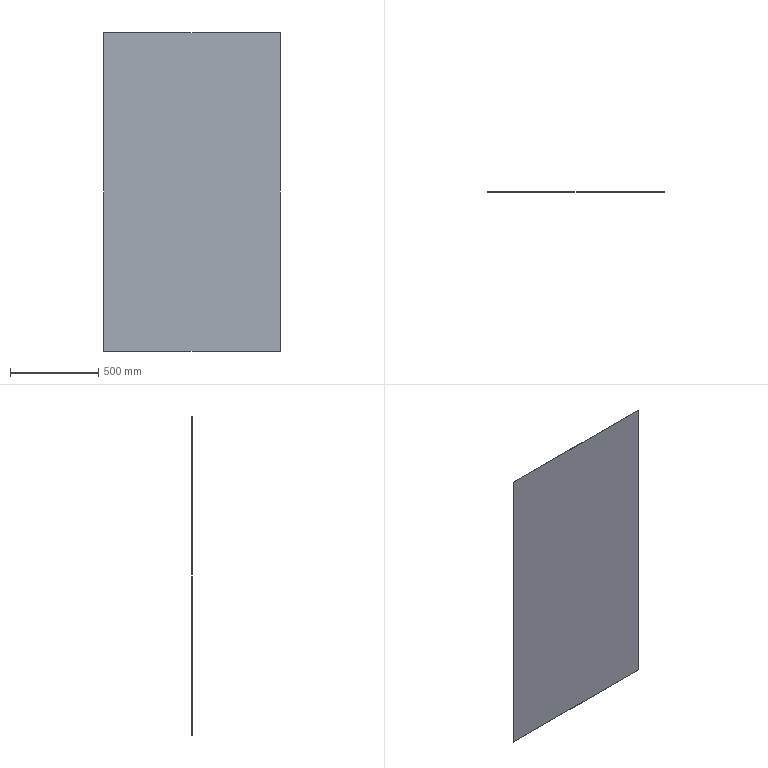Part | SolidWorks | features Extrusion 1 | 1 solid | 6 faces | box 1000 x 1 x 1800 mm | volume 1800000 mm3 | plane 6
STEP:
#1=CARTESIAN_POINT('',(500.,0.,900.));
#2=VERTEX_POINT('',#1);
#3=CARTESIAN_POINT('',(500.,0.,-900.));
#4=VERTEX_POINT('',#3);
#5=CARTESIAN_POINT('',(500.,0.,900.));
#6=DIRECTION('',(0.,0.,-1.));
#7=VECTOR('',#6,1000.);
#8=LINE('',#5,#7);
#9=EDGE_CURVE('',#2,#4,#8,.T.);
#10=ORIENTED_EDGE('',*,*,#9,.T.);
#11=CARTESIAN_POINT('',(500.,1.,-900.));
#12=VERTEX_POINT('',#11);
#13=CARTESIAN_POINT('',(500.,1.,-900.));
#14=DIRECTION('',(0.,-1.,0.));
#15=VECTOR('',#14,1000.);
#16=LINE('',#13,#15);
#17=EDGE_CURVE('',#12,#4,#16,.T.);
#18=ORIENTED_EDGE('',*,*,#17,.F.);
#19=CARTESIAN_POINT('',(500.,1.,900.));
#20=VERTEX_POINT('',#19);
#21=CARTESIAN_POINT('',(500.,1.,900.));
#22=DIRECTION('',(0.,0.,-1.));
#23=VECTOR('',#22,1000.);
#24=LINE('',#21,#23);
#25=EDGE_CURVE('',#20,#12,#24,.T.);
#26=ORIENTED_EDGE('',*,*,#25,.F.);
#27=CARTESIAN_POINT('',(500.,1.,900.));
#28=DIRECTION('',(0.,-1.,0.));
#29=VECTOR('',#28,1000.);
#30=LINE('',#27,#29);
#31=EDGE_CURVE('',#20,#2,#30,.T.);
#32=ORIENTED_EDGE('',*,*,#31,.T.);
#33=EDGE_LOOP('',(#10,#18,#26,#32));
#34=FACE_OUTER_BOUND('',#33,.T.);
#35=CARTESIAN_POINT('',(500.,1.,900.));
#36=DIRECTION('',(-1.,0.,0.));
#37=DIRECTION('',(0.,0.,1.));
#38=AXIS2_PLACEMENT_3D('',#35,#36,#37);
#39=PLANE('',#38);
#40=ADVANCED_FACE('',(#34),#39,.F.);
#41=CARTESIAN_POINT('',(-500.,0.,-900.));
#42=VERTEX_POINT('',#41);
#43=CARTESIAN_POINT('',(-500.,0.,-900.));
#44=DIRECTION('',(-1.,0.,0.));
#45=VECTOR('',#44,1000.);
#46=LINE('',#43,#45);
#47=EDGE_CURVE('',#4,#42,#46,.T.);
#48=ORIENTED_EDGE('',*,*,#47,.T.);
#49=CARTESIAN_POINT('',(-500.,1.,-900.));
#50=VERTEX_POINT('',#49);
#51=CARTESIAN_POINT('',(-500.,1.,-900.));
#52=DIRECTION('',(0.,-1.,0.));
#53=VECTOR('',#52,1000.);
#54=LINE('',#51,#53);
#55=EDGE_CURVE('',#50,#42,#54,.T.);
#56=ORIENTED_EDGE('',*,*,#55,.F.);
#57=CARTESIAN_POINT('',(-500.,1.,-900.));
#58=DIRECTION('',(-1.,0.,0.));
#59=VECTOR('',#58,1000.);
#60=LINE('',#57,#59);
#61=EDGE_CURVE('',#12,#50,#60,.T.);
#62=ORIENTED_EDGE('',*,*,#61,.F.);
#63=ORIENTED_EDGE('',*,*,#17,.T.);
#64=EDGE_LOOP('',(#48,#56,#62,#63));
#65=FACE_OUTER_BOUND('',#64,.T.);
#66=CARTESIAN_POINT('',(-500.,1.,-900.));
#67=DIRECTION('',(0.,0.,1.));
#68=DIRECTION('',(1.,0.,0.));
#69=AXIS2_PLACEMENT_3D('',#66,#67,#68);
#70=PLANE('',#69);
#71=ADVANCED_FACE('',(#65),#70,.F.);
#72=CARTESIAN_POINT('',(-500.,0.,900.));
#73=VERTEX_POINT('',#72);
#74=CARTESIAN_POINT('',(-500.,0.,900.));
#75=DIRECTION('',(0.,0.,1.));
#76=VECTOR('',#75,1000.);
#77=LINE('',#74,#76);
#78=EDGE_CURVE('',#42,#73,#77,.T.);
#79=ORIENTED_EDGE('',*,*,#78,.T.);
#80=CARTESIAN_POINT('',(-500.,1.,900.));
#81=VERTEX_POINT('',#80);
#82=CARTESIAN_POINT('',(-500.,1.,900.));
#83=DIRECTION('',(0.,-1.,0.));
#84=VECTOR('',#83,1000.);
#85=LINE('',#82,#84);
#86=EDGE_CURVE('',#81,#73,#85,.T.);
#87=ORIENTED_EDGE('',*,*,#86,.F.);
#88=CARTESIAN_POINT('',(-500.,1.,900.));
#89=DIRECTION('',(0.,0.,1.));
#90=VECTOR('',#89,1000.);
#91=LINE('',#88,#90);
#92=EDGE_CURVE('',#50,#81,#91,.T.);
#93=ORIENTED_EDGE('',*,*,#92,.F.);
#94=ORIENTED_EDGE('',*,*,#55,.T.);
#95=EDGE_LOOP('',(#79,#87,#93,#94));
#96=FACE_OUTER_BOUND('',#95,.T.);
#97=CARTESIAN_POINT('',(-500.,1.,900.));
#98=DIRECTION('',(1.,0.,0.));
#99=DIRECTION('',(0.,0.,-1.));
#100=AXIS2_PLACEMENT_3D('',#97,#98,#99);
#101=PLANE('',#100);
#102=ADVANCED_FACE('',(#96),#101,.F.);
#103=CARTESIAN_POINT('',(-500.,0.,900.));
#104=DIRECTION('',(1.,0.,0.));
#105=VECTOR('',#104,1000.);
#106=LINE('',#103,#105);
#107=EDGE_CURVE('',#73,#2,#106,.T.);
#108=ORIENTED_EDGE('',*,*,#107,.T.);
#109=ORIENTED_EDGE('',*,*,#31,.F.);
#110=CARTESIAN_POINT('',(-500.,1.,900.));
#111=DIRECTION('',(1.,0.,0.));
#112=VECTOR('',#111,1000.);
#113=LINE('',#110,#112);
#114=EDGE_CURVE('',#81,#20,#113,.T.);
#115=ORIENTED_EDGE('',*,*,#114,.F.);
#116=ORIENTED_EDGE('',*,*,#86,.T.);
#117=EDGE_LOOP('',(#108,#109,#115,#116));
#118=FACE_OUTER_BOUND('',#117,.T.);
#119=CARTESIAN_POINT('',(-500.,1.,900.));
#120=DIRECTION('',(0.,0.,-1.));
#121=DIRECTION('',(-1.,0.,0.));
#122=AXIS2_PLACEMENT_3D('',#119,#120,#121);
#123=PLANE('',#122);
#124=ADVANCED_FACE('',(#118),#123,.F.);
#125=ORIENTED_EDGE('',*,*,#25,.T.);
#126=ORIENTED_EDGE('',*,*,#61,.T.);
#127=ORIENTED_EDGE('',*,*,#92,.T.);
#128=ORIENTED_EDGE('',*,*,#114,.T.);
#129=EDGE_LOOP('',(#125,#126,#127,#128));
#130=FACE_OUTER_BOUND('',#129,.T.);
#131=CARTESIAN_POINT('',(0.,1.,0.));
#132=DIRECTION('',(0.,-1.,0.));
#133=DIRECTION('',(0.,0.,-1.));
#134=AXIS2_PLACEMENT_3D('',#131,#132,#133);
#135=PLANE('',#134);
#136=ADVANCED_FACE('',(#130),#135,.F.);
#137=ORIENTED_EDGE('',*,*,#9,.F.);
#138=ORIENTED_EDGE('',*,*,#107,.F.);
#139=ORIENTED_EDGE('',*,*,#78,.F.);
#140=ORIENTED_EDGE('',*,*,#47,.F.);
#141=EDGE_LOOP('',(#137,#138,#139,#140));
#142=FACE_OUTER_BOUND('',#141,.T.);
#143=CARTESIAN_POINT('',(0.,0.,0.));
#144=DIRECTION('',(0.,-1.,0.));
#145=DIRECTION('',(0.,0.,-1.));
#146=AXIS2_PLACEMENT_3D('',#143,#144,#145);
#147=PLANE('',#146);
#148=ADVANCED_FACE('',(#142),#147,.T.);
#149=CLOSED_SHELL('',(#40,#71,#102,#124,#136,#148));
#150=MANIFOLD_SOLID_BREP('',#149);
#151=CARTESIAN_POINT('',(0.,0.,0.));
#152=DIRECTION('',(0.,0.,1.));
#153=DIRECTION('',(1.,0.,0.));
#154=AXIS2_PLACEMENT_3D('',#151,#152,#153);
#155=(LENGTH_UNIT()NAMED_UNIT(*)SI_UNIT(.MILLI.,.METRE.));
#156=UNCERTAINTY_MEASURE_WITH_UNIT(LENGTH_MEASURE(0.00001),#155,'','');
#157=(NAMED_UNIT(*)PLANE_ANGLE_UNIT()SI_UNIT($,.RADIAN.));
#158=(NAMED_UNIT(*)SI_UNIT($,.STERADIAN.)SOLID_ANGLE_UNIT());
#159=(GEOMETRIC_REPRESENTATION_CONTEXT(3)GLOBAL_UNCERTAINTY_ASSIGNED_CONTEXT((#156))GLOBAL_UNIT_ASSIGNED_CONTEXT((#155,#157,#158))REPRESENTATION_CONTEXT('',''));
#160=ADVANCED_BREP_SHAPE_REPRESENTATION('',(#150,#154),#159);